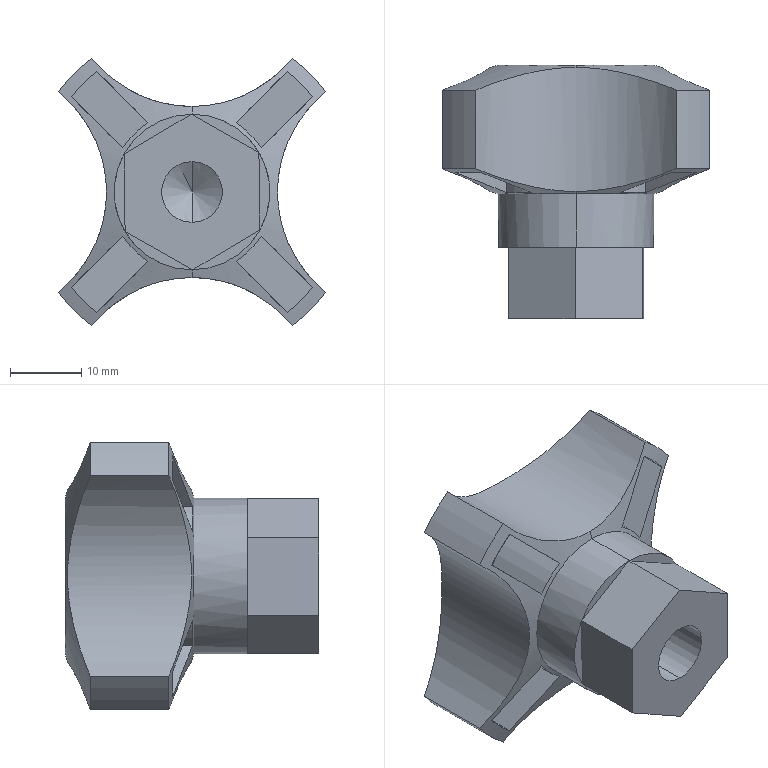Part | SolidWorks | features BaseBody 1 | 1 solid | 53 faces | box 37.452 x 35.5 x 37.452 mm | volume 16341 mm3 | plane 26 | cylinder 21 | cone 6 | commonest cylinder face diameters 36 x5 23 x4 43 x4 46.8 x4 8.5 x2 21.8 x2